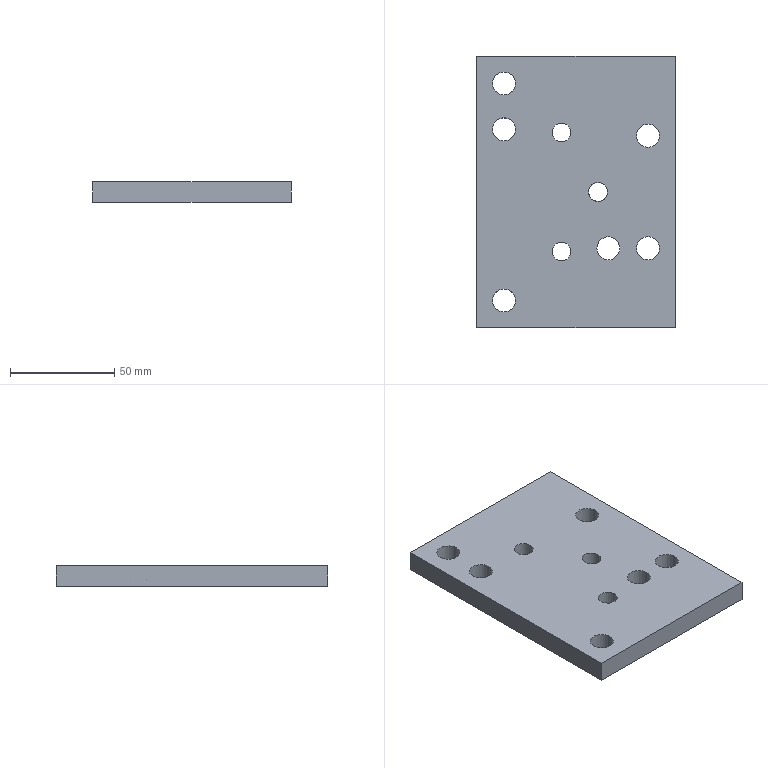Part | STEP file | PN_0042_id870_x_t | 1 solid | 15 faces | box 95 x 130 x 10 mm | volume 115889 mm3 | cylinder 9 | plane 6 | commonest cylinder face diameters 11 x6 9 x3
STEP:
#1=CARTESIAN_POINT('',(-190.55,-65.,105.));
#2=VERTEX_POINT('',#1);
#3=CARTESIAN_POINT('',(-190.55,65.,105.));
#4=VERTEX_POINT('',#3);
#5=CARTESIAN_POINT('',(-190.55,64.,105.));
#6=DIRECTION('',(0.,1.,0.));
#7=VECTOR('',#6,1.);
#8=LINE('',#5,#7);
#9=EDGE_CURVE('',#2,#4,#8,.T.);
#10=ORIENTED_EDGE('',*,*,#9,.F.);
#11=CARTESIAN_POINT('',(-190.55,-65.,95.));
#12=VERTEX_POINT('',#11);
#13=CARTESIAN_POINT('',(-190.55,-65.,95.));
#14=DIRECTION('',(0.,0.,1.));
#15=VECTOR('',#14,1.);
#16=LINE('',#13,#15);
#17=EDGE_CURVE('',#12,#2,#16,.T.);
#18=ORIENTED_EDGE('',*,*,#17,.F.);
#19=CARTESIAN_POINT('',(-190.55,65.,95.));
#20=VERTEX_POINT('',#19);
#21=CARTESIAN_POINT('',(-190.55,0.,95.));
#22=DIRECTION('',(0.,1.,0.));
#23=VECTOR('',#22,1.);
#24=LINE('',#21,#23);
#25=EDGE_CURVE('',#12,#20,#24,.T.);
#26=ORIENTED_EDGE('',*,*,#25,.T.);
#27=CARTESIAN_POINT('',(-190.55,65.,95.));
#28=DIRECTION('',(0.,0.,-1.));
#29=VECTOR('',#28,1.);
#30=LINE('',#27,#29);
#31=EDGE_CURVE('',#4,#20,#30,.T.);
#32=ORIENTED_EDGE('',*,*,#31,.F.);
#33=EDGE_LOOP('',(#10,#18,#26,#32));
#34=FACE_OUTER_BOUND('',#33,.T.);
#35=CARTESIAN_POINT('',(-190.55,0.,95.));
#36=DIRECTION('',(1.,0.,0.));
#37=DIRECTION('',(0.,1.,0.));
#38=AXIS2_PLACEMENT_3D('',#35,#36,#37);
#39=PLANE('',#38);
#40=ADVANCED_FACE('',(#34),#39,.T.);
#41=CARTESIAN_POINT('',(-285.55,-65.,95.));
#42=VERTEX_POINT('',#41);
#43=CARTESIAN_POINT('',(-224.,-65.,95.));
#44=DIRECTION('',(1.,0.,0.));
#45=VECTOR('',#44,1.);
#46=LINE('',#43,#45);
#47=EDGE_CURVE('',#42,#12,#46,.T.);
#48=ORIENTED_EDGE('',*,*,#47,.T.);
#49=ORIENTED_EDGE('',*,*,#17,.T.);
#50=CARTESIAN_POINT('',(-285.55,-65.,105.));
#51=VERTEX_POINT('',#50);
#52=CARTESIAN_POINT('',(-224.,-65.,105.));
#53=DIRECTION('',(1.,0.,0.));
#54=VECTOR('',#53,1.);
#55=LINE('',#52,#54);
#56=EDGE_CURVE('',#51,#2,#55,.T.);
#57=ORIENTED_EDGE('',*,*,#56,.F.);
#58=CARTESIAN_POINT('',(-285.55,-65.,95.));
#59=DIRECTION('',(0.,0.,1.));
#60=VECTOR('',#59,1.);
#61=LINE('',#58,#60);
#62=EDGE_CURVE('',#42,#51,#61,.T.);
#63=ORIENTED_EDGE('',*,*,#62,.F.);
#64=EDGE_LOOP('',(#48,#49,#57,#63));
#65=FACE_OUTER_BOUND('',#64,.T.);
#66=CARTESIAN_POINT('',(-224.,-65.,95.));
#67=DIRECTION('',(0.,1.,0.));
#68=DIRECTION('',(-1.,0.,0.));
#69=AXIS2_PLACEMENT_3D('',#66,#67,#68);
#70=PLANE('',#69);
#71=ADVANCED_FACE('',(#65),#70,.F.);
#72=ORIENTED_EDGE('',*,*,#9,.T.);
#73=CARTESIAN_POINT('',(-285.55,65.,105.));
#74=VERTEX_POINT('',#73);
#75=CARTESIAN_POINT('',(-119.811,65.,105.));
#76=DIRECTION('',(1.,0.,0.));
#77=VECTOR('',#76,1.);
#78=LINE('',#75,#77);
#79=EDGE_CURVE('',#74,#4,#78,.T.);
#80=ORIENTED_EDGE('',*,*,#79,.F.);
#81=CARTESIAN_POINT('',(-285.55,0.,105.));
#82=DIRECTION('',(0.,-1.,0.));
#83=VECTOR('',#82,1.);
#84=LINE('',#81,#83);
#85=EDGE_CURVE('',#74,#51,#84,.T.);
#86=ORIENTED_EDGE('',*,*,#85,.T.);
#87=ORIENTED_EDGE('',*,*,#56,.T.);
#88=EDGE_LOOP('',(#72,#80,#86,#87));
#89=FACE_BOUND('',#88,.T.);
#90=CARTESIAN_POINT('',(-228.05,-27.,105.));
#91=VERTEX_POINT('',#90);
#92=CARTESIAN_POINT('',(-222.55,-27.,105.));
#93=DIRECTION('',(0.,0.,-1.));
#94=DIRECTION('',(-1.,0.,0.));
#95=AXIS2_PLACEMENT_3D('',#92,#93,#94);
#96=CIRCLE('',#95,5.5);
#97=EDGE_CURVE('',#91,#91,#96,.T.);
#98=ORIENTED_EDGE('',*,*,#97,.T.);
#99=EDGE_LOOP('',(#98));
#100=FACE_BOUND('',#99,.T.);
#101=CARTESIAN_POINT('',(-278.05,30.,105.));
#102=VERTEX_POINT('',#101);
#103=CARTESIAN_POINT('',(-272.55,30.,105.));
#104=DIRECTION('',(0.,0.,-1.));
#105=DIRECTION('',(-1.,0.,0.));
#106=AXIS2_PLACEMENT_3D('',#103,#104,#105);
#107=CIRCLE('',#106,5.5);
#108=EDGE_CURVE('',#102,#102,#107,.T.);
#109=ORIENTED_EDGE('',*,*,#108,.T.);
#110=EDGE_LOOP('',(#109));
#111=FACE_BOUND('',#110,.T.);
#112=CARTESIAN_POINT('',(-278.05,52.,105.));
#113=VERTEX_POINT('',#112);
#114=CARTESIAN_POINT('',(-272.55,52.,105.));
#115=DIRECTION('',(0.,0.,-1.));
#116=DIRECTION('',(-1.,0.,0.));
#117=AXIS2_PLACEMENT_3D('',#114,#115,#116);
#118=CIRCLE('',#117,5.5);
#119=EDGE_CURVE('',#113,#113,#118,.T.);
#120=ORIENTED_EDGE('',*,*,#119,.T.);
#121=EDGE_LOOP('',(#120));
#122=FACE_BOUND('',#121,.T.);
#123=CARTESIAN_POINT('',(-278.05,-52.,105.));
#124=VERTEX_POINT('',#123);
#125=CARTESIAN_POINT('',(-272.55,-52.,105.));
#126=DIRECTION('',(0.,0.,1.));
#127=DIRECTION('',(-1.,0.,0.));
#128=AXIS2_PLACEMENT_3D('',#125,#126,#127);
#129=CIRCLE('',#128,5.5);
#130=EDGE_CURVE('',#124,#124,#129,.T.);
#131=ORIENTED_EDGE('',*,*,#130,.F.);
#132=EDGE_LOOP('',(#131));
#133=FACE_BOUND('',#132,.T.);
#134=CARTESIAN_POINT('',(-209.05,-27.,105.));
#135=VERTEX_POINT('',#134);
#136=CARTESIAN_POINT('',(-203.55,-27.,105.));
#137=DIRECTION('',(0.,0.,1.));
#138=DIRECTION('',(-1.,0.,0.));
#139=AXIS2_PLACEMENT_3D('',#136,#137,#138);
#140=CIRCLE('',#139,5.5);
#141=EDGE_CURVE('',#135,#135,#140,.T.);
#142=ORIENTED_EDGE('',*,*,#141,.F.);
#143=EDGE_LOOP('',(#142));
#144=FACE_BOUND('',#143,.T.);
#145=CARTESIAN_POINT('',(-209.05,27.,105.));
#146=VERTEX_POINT('',#145);
#147=CARTESIAN_POINT('',(-203.55,27.,105.));
#148=DIRECTION('',(0.,0.,-1.));
#149=DIRECTION('',(-1.,0.,0.));
#150=AXIS2_PLACEMENT_3D('',#147,#148,#149);
#151=CIRCLE('',#150,5.5);
#152=EDGE_CURVE('',#146,#146,#151,.T.);
#153=ORIENTED_EDGE('',*,*,#152,.T.);
#154=EDGE_LOOP('',(#153));
#155=FACE_BOUND('',#154,.T.);
#156=CARTESIAN_POINT('',(-227.5,4.5,105.));
#157=VERTEX_POINT('',#156);
#158=CARTESIAN_POINT('',(-227.5,0.,105.));
#159=DIRECTION('',(0.,0.,-1.));
#160=DIRECTION('',(0.,1.,0.));
#161=AXIS2_PLACEMENT_3D('',#158,#159,#160);
#162=CIRCLE('',#161,4.5);
#163=EDGE_CURVE('',#157,#157,#162,.T.);
#164=ORIENTED_EDGE('',*,*,#163,.T.);
#165=EDGE_LOOP('',(#164));
#166=FACE_BOUND('',#165,.T.);
#167=CARTESIAN_POINT('',(-249.5,-28.5,105.));
#168=VERTEX_POINT('',#167);
#169=CARTESIAN_POINT('',(-245.,-28.5,105.));
#170=DIRECTION('',(0.,0.,1.));
#171=DIRECTION('',(-1.,0.,0.));
#172=AXIS2_PLACEMENT_3D('',#169,#170,#171);
#173=CIRCLE('',#172,4.5);
#174=EDGE_CURVE('',#168,#168,#173,.T.);
#175=ORIENTED_EDGE('',*,*,#174,.F.);
#176=EDGE_LOOP('',(#175));
#177=FACE_BOUND('',#176,.T.);
#178=CARTESIAN_POINT('',(-249.5,28.5,105.));
#179=VERTEX_POINT('',#178);
#180=CARTESIAN_POINT('',(-245.,28.5,105.));
#181=DIRECTION('',(0.,0.,-1.));
#182=DIRECTION('',(-1.,0.,0.));
#183=AXIS2_PLACEMENT_3D('',#180,#181,#182);
#184=CIRCLE('',#183,4.5);
#185=EDGE_CURVE('',#179,#179,#184,.T.);
#186=ORIENTED_EDGE('',*,*,#185,.T.);
#187=EDGE_LOOP('',(#186));
#188=FACE_BOUND('',#187,.T.);
#189=CARTESIAN_POINT('',(-119.811,64.,105.));
#190=DIRECTION('',(0.,0.,1.));
#191=DIRECTION('',(1.,0.,0.));
#192=AXIS2_PLACEMENT_3D('',#189,#190,#191);
#193=PLANE('',#192);
#194=ADVANCED_FACE('',(#89,#100,#111,#122,#133,#144,#155,#166,#177,#188),#193,.T.);
#195=ORIENTED_EDGE('',*,*,#25,.F.);
#196=ORIENTED_EDGE('',*,*,#47,.F.);
#197=CARTESIAN_POINT('',(-285.55,65.,95.));
#198=VERTEX_POINT('',#197);
#199=CARTESIAN_POINT('',(-285.55,0.,95.));
#200=DIRECTION('',(0.,-1.,0.));
#201=VECTOR('',#200,1.);
#202=LINE('',#199,#201);
#203=EDGE_CURVE('',#198,#42,#202,.T.);
#204=ORIENTED_EDGE('',*,*,#203,.F.);
#205=CARTESIAN_POINT('',(-119.811,65.,95.));
#206=DIRECTION('',(1.,0.,0.));
#207=VECTOR('',#206,1.);
#208=LINE('',#205,#207);
#209=EDGE_CURVE('',#198,#20,#208,.T.);
#210=ORIENTED_EDGE('',*,*,#209,.T.);
#211=EDGE_LOOP('',(#195,#196,#204,#210));
#212=FACE_BOUND('',#211,.T.);
#213=CARTESIAN_POINT('',(-228.05,-27.,95.));
#214=VERTEX_POINT('',#213);
#215=CARTESIAN_POINT('',(-222.55,-27.,95.));
#216=DIRECTION('',(0.,0.,1.));
#217=DIRECTION('',(-1.,0.,0.));
#218=AXIS2_PLACEMENT_3D('',#215,#216,#217);
#219=CIRCLE('',#218,5.5);
#220=EDGE_CURVE('',#214,#214,#219,.T.);
#221=ORIENTED_EDGE('',*,*,#220,.T.);
#222=EDGE_LOOP('',(#221));
#223=FACE_BOUND('',#222,.T.);
#224=CARTESIAN_POINT('',(-278.05,30.,95.));
#225=VERTEX_POINT('',#224);
#226=CARTESIAN_POINT('',(-272.55,30.,95.));
#227=DIRECTION('',(0.,0.,1.));
#228=DIRECTION('',(-1.,0.,0.));
#229=AXIS2_PLACEMENT_3D('',#226,#227,#228);
#230=CIRCLE('',#229,5.5);
#231=EDGE_CURVE('',#225,#225,#230,.T.);
#232=ORIENTED_EDGE('',*,*,#231,.T.);
#233=EDGE_LOOP('',(#232));
#234=FACE_BOUND('',#233,.T.);
#235=CARTESIAN_POINT('',(-267.05,52.,95.));
#236=VERTEX_POINT('',#235);
#237=CARTESIAN_POINT('',(-272.55,52.,95.));
#238=DIRECTION('',(0.,0.,-1.));
#239=DIRECTION('',(1.,0.,0.));
#240=AXIS2_PLACEMENT_3D('',#237,#238,#239);
#241=CIRCLE('',#240,5.5);
#242=EDGE_CURVE('',#236,#236,#241,.T.);
#243=ORIENTED_EDGE('',*,*,#242,.F.);
#244=EDGE_LOOP('',(#243));
#245=FACE_BOUND('',#244,.T.);
#246=CARTESIAN_POINT('',(-267.05,-52.,95.));
#247=VERTEX_POINT('',#246);
#248=CARTESIAN_POINT('',(-272.55,-52.,95.));
#249=DIRECTION('',(0.,0.,-1.));
#250=DIRECTION('',(1.,0.,0.));
#251=AXIS2_PLACEMENT_3D('',#248,#249,#250);
#252=CIRCLE('',#251,5.5);
#253=EDGE_CURVE('',#247,#247,#252,.T.);
#254=ORIENTED_EDGE('',*,*,#253,.F.);
#255=EDGE_LOOP('',(#254));
#256=FACE_BOUND('',#255,.T.);
#257=CARTESIAN_POINT('',(-198.05,-27.,95.));
#258=VERTEX_POINT('',#257);
#259=CARTESIAN_POINT('',(-203.55,-27.,95.));
#260=DIRECTION('',(0.,0.,-1.));
#261=DIRECTION('',(1.,0.,0.));
#262=AXIS2_PLACEMENT_3D('',#259,#260,#261);
#263=CIRCLE('',#262,5.5);
#264=EDGE_CURVE('',#258,#258,#263,.T.);
#265=ORIENTED_EDGE('',*,*,#264,.F.);
#266=EDGE_LOOP('',(#265));
#267=FACE_BOUND('',#266,.T.);
#268=CARTESIAN_POINT('',(-198.05,27.,95.));
#269=VERTEX_POINT('',#268);
#270=CARTESIAN_POINT('',(-203.55,27.,95.));
#271=DIRECTION('',(0.,0.,-1.));
#272=DIRECTION('',(1.,0.,0.));
#273=AXIS2_PLACEMENT_3D('',#270,#271,#272);
#274=CIRCLE('',#273,5.5);
#275=EDGE_CURVE('',#269,#269,#274,.T.);
#276=ORIENTED_EDGE('',*,*,#275,.F.);
#277=EDGE_LOOP('',(#276));
#278=FACE_BOUND('',#277,.T.);
#279=CARTESIAN_POINT('',(-223.,0.,95.));
#280=VERTEX_POINT('',#279);
#281=CARTESIAN_POINT('',(-227.5,0.,95.));
#282=DIRECTION('',(0.,0.,-1.));
#283=DIRECTION('',(1.,0.,0.));
#284=AXIS2_PLACEMENT_3D('',#281,#282,#283);
#285=CIRCLE('',#284,4.5);
#286=EDGE_CURVE('',#280,#280,#285,.T.);
#287=ORIENTED_EDGE('',*,*,#286,.F.);
#288=EDGE_LOOP('',(#287));
#289=FACE_BOUND('',#288,.T.);
#290=CARTESIAN_POINT('',(-240.5,-28.5,95.));
#291=VERTEX_POINT('',#290);
#292=CARTESIAN_POINT('',(-245.,-28.5,95.));
#293=DIRECTION('',(0.,0.,-1.));
#294=DIRECTION('',(1.,0.,0.));
#295=AXIS2_PLACEMENT_3D('',#292,#293,#294);
#296=CIRCLE('',#295,4.5);
#297=EDGE_CURVE('',#291,#291,#296,.T.);
#298=ORIENTED_EDGE('',*,*,#297,.F.);
#299=EDGE_LOOP('',(#298));
#300=FACE_BOUND('',#299,.T.);
#301=CARTESIAN_POINT('',(-240.5,28.5,95.));
#302=VERTEX_POINT('',#301);
#303=CARTESIAN_POINT('',(-245.,28.5,95.));
#304=DIRECTION('',(0.,0.,-1.));
#305=DIRECTION('',(1.,0.,0.));
#306=AXIS2_PLACEMENT_3D('',#303,#304,#305);
#307=CIRCLE('',#306,4.5);
#308=EDGE_CURVE('',#302,#302,#307,.T.);
#309=ORIENTED_EDGE('',*,*,#308,.F.);
#310=EDGE_LOOP('',(#309));
#311=FACE_BOUND('',#310,.T.);
#312=CARTESIAN_POINT('',(-119.811,64.,95.));
#313=DIRECTION('',(0.,0.,1.));
#314=DIRECTION('',(1.,0.,0.));
#315=AXIS2_PLACEMENT_3D('',#312,#313,#314);
#316=PLANE('',#315);
#317=ADVANCED_FACE('',(#212,#223,#234,#245,#256,#267,#278,#289,#300,#311),#316,.F.);
#318=CARTESIAN_POINT('',(-285.55,65.,95.));
#319=DIRECTION('',(0.,0.,1.));
#320=VECTOR('',#319,1.);
#321=LINE('',#318,#320);
#322=EDGE_CURVE('',#198,#74,#321,.T.);
#323=ORIENTED_EDGE('',*,*,#322,.F.);
#324=ORIENTED_EDGE('',*,*,#203,.T.);
#325=ORIENTED_EDGE('',*,*,#62,.T.);
#326=ORIENTED_EDGE('',*,*,#85,.F.);
#327=EDGE_LOOP('',(#323,#324,#325,#326));
#328=FACE_OUTER_BOUND('',#327,.T.);
#329=CARTESIAN_POINT('',(-285.55,0.,95.));
#330=DIRECTION('',(1.,0.,0.));
#331=DIRECTION('',(0.,1.,0.));
#332=AXIS2_PLACEMENT_3D('',#329,#330,#331);
#333=PLANE('',#332);
#334=ADVANCED_FACE('',(#328),#333,.F.);
#335=ORIENTED_EDGE('',*,*,#79,.T.);
#336=ORIENTED_EDGE('',*,*,#31,.T.);
#337=ORIENTED_EDGE('',*,*,#209,.F.);
#338=ORIENTED_EDGE('',*,*,#322,.T.);
#339=EDGE_LOOP('',(#335,#336,#337,#338));
#340=FACE_OUTER_BOUND('',#339,.T.);
#341=CARTESIAN_POINT('',(-119.811,65.,95.));
#342=DIRECTION('',(0.,-1.,0.));
#343=DIRECTION('',(1.,0.,0.));
#344=AXIS2_PLACEMENT_3D('',#341,#342,#343);
#345=PLANE('',#344);
#346=ADVANCED_FACE('',(#340),#345,.F.);
#347=ORIENTED_EDGE('',*,*,#308,.T.);
#348=EDGE_LOOP('',(#347));
#349=FACE_BOUND('',#348,.T.);
#350=ORIENTED_EDGE('',*,*,#185,.F.);
#351=EDGE_LOOP('',(#350));
#352=FACE_BOUND('',#351,.T.);
#353=CARTESIAN_POINT('',(-245.,28.5,105.));
#354=DIRECTION('',(0.,0.,-1.));
#355=DIRECTION('',(-1.,0.,0.));
#356=AXIS2_PLACEMENT_3D('',#353,#354,#355);
#357=CYLINDRICAL_SURFACE('',#356,4.5);
#358=ADVANCED_FACE('',(#349,#352),#357,.F.);
#359=ORIENTED_EDGE('',*,*,#297,.T.);
#360=EDGE_LOOP('',(#359));
#361=FACE_BOUND('',#360,.T.);
#362=ORIENTED_EDGE('',*,*,#174,.T.);
#363=EDGE_LOOP('',(#362));
#364=FACE_BOUND('',#363,.T.);
#365=CARTESIAN_POINT('',(-245.,-28.5,105.));
#366=DIRECTION('',(0.,0.,-1.));
#367=DIRECTION('',(-1.,0.,0.));
#368=AXIS2_PLACEMENT_3D('',#365,#366,#367);
#369=CYLINDRICAL_SURFACE('',#368,4.5);
#370=ADVANCED_FACE('',(#361,#364),#369,.F.);
#371=ORIENTED_EDGE('',*,*,#286,.T.);
#372=EDGE_LOOP('',(#371));
#373=FACE_BOUND('',#372,.T.);
#374=ORIENTED_EDGE('',*,*,#163,.F.);
#375=EDGE_LOOP('',(#374));
#376=FACE_BOUND('',#375,.T.);
#377=CARTESIAN_POINT('',(-227.5,0.,105.));
#378=DIRECTION('',(0.,0.,-1.));
#379=DIRECTION('',(0.,1.,0.));
#380=AXIS2_PLACEMENT_3D('',#377,#378,#379);
#381=CYLINDRICAL_SURFACE('',#380,4.5);
#382=ADVANCED_FACE('',(#373,#376),#381,.F.);
#383=ORIENTED_EDGE('',*,*,#275,.T.);
#384=EDGE_LOOP('',(#383));
#385=FACE_BOUND('',#384,.T.);
#386=ORIENTED_EDGE('',*,*,#152,.F.);
#387=EDGE_LOOP('',(#386));
#388=FACE_BOUND('',#387,.T.);
#389=CARTESIAN_POINT('',(-203.55,27.,105.));
#390=DIRECTION('',(0.,0.,-1.));
#391=DIRECTION('',(-1.,0.,0.));
#392=AXIS2_PLACEMENT_3D('',#389,#390,#391);
#393=CYLINDRICAL_SURFACE('',#392,5.5);
#394=ADVANCED_FACE('',(#385,#388),#393,.F.);
#395=ORIENTED_EDGE('',*,*,#264,.T.);
#396=EDGE_LOOP('',(#395));
#397=FACE_BOUND('',#396,.T.);
#398=ORIENTED_EDGE('',*,*,#141,.T.);
#399=EDGE_LOOP('',(#398));
#400=FACE_BOUND('',#399,.T.);
#401=CARTESIAN_POINT('',(-203.55,-27.,105.));
#402=DIRECTION('',(0.,0.,-1.));
#403=DIRECTION('',(-1.,0.,0.));
#404=AXIS2_PLACEMENT_3D('',#401,#402,#403);
#405=CYLINDRICAL_SURFACE('',#404,5.5);
#406=ADVANCED_FACE('',(#397,#400),#405,.F.);
#407=ORIENTED_EDGE('',*,*,#253,.T.);
#408=EDGE_LOOP('',(#407));
#409=FACE_BOUND('',#408,.T.);
#410=ORIENTED_EDGE('',*,*,#130,.T.);
#411=EDGE_LOOP('',(#410));
#412=FACE_BOUND('',#411,.T.);
#413=CARTESIAN_POINT('',(-272.55,-52.,105.));
#414=DIRECTION('',(0.,0.,-1.));
#415=DIRECTION('',(-1.,0.,0.));
#416=AXIS2_PLACEMENT_3D('',#413,#414,#415);
#417=CYLINDRICAL_SURFACE('',#416,5.5);
#418=ADVANCED_FACE('',(#409,#412),#417,.F.);
#419=ORIENTED_EDGE('',*,*,#242,.T.);
#420=EDGE_LOOP('',(#419));
#421=FACE_BOUND('',#420,.T.);
#422=ORIENTED_EDGE('',*,*,#119,.F.);
#423=EDGE_LOOP('',(#422));
#424=FACE_BOUND('',#423,.T.);
#425=CARTESIAN_POINT('',(-272.55,52.,105.));
#426=DIRECTION('',(0.,0.,-1.));
#427=DIRECTION('',(-1.,0.,0.));
#428=AXIS2_PLACEMENT_3D('',#425,#426,#427);
#429=CYLINDRICAL_SURFACE('',#428,5.5);
#430=ADVANCED_FACE('',(#421,#424),#429,.F.);
#431=ORIENTED_EDGE('',*,*,#231,.F.);
#432=EDGE_LOOP('',(#431));
#433=FACE_BOUND('',#432,.T.);
#434=ORIENTED_EDGE('',*,*,#108,.F.);
#435=EDGE_LOOP('',(#434));
#436=FACE_BOUND('',#435,.T.);
#437=CARTESIAN_POINT('',(-272.55,30.,105.));
#438=DIRECTION('',(0.,0.,-1.));
#439=DIRECTION('',(-1.,0.,0.));
#440=AXIS2_PLACEMENT_3D('',#437,#438,#439);
#441=CYLINDRICAL_SURFACE('',#440,5.5);
#442=ADVANCED_FACE('',(#433,#436),#441,.F.);
#443=ORIENTED_EDGE('',*,*,#220,.F.);
#444=EDGE_LOOP('',(#443));
#445=FACE_BOUND('',#444,.T.);
#446=ORIENTED_EDGE('',*,*,#97,.F.);
#447=EDGE_LOOP('',(#446));
#448=FACE_BOUND('',#447,.T.);
#449=CARTESIAN_POINT('',(-222.55,-27.,105.));
#450=DIRECTION('',(0.,0.,-1.));
#451=DIRECTION('',(-1.,0.,0.));
#452=AXIS2_PLACEMENT_3D('',#449,#450,#451);
#453=CYLINDRICAL_SURFACE('',#452,5.5);
#454=ADVANCED_FACE('',(#445,#448),#453,.F.);
#455=CLOSED_SHELL('',(#40,#71,#194,#317,#334,#346,#358,#370,#382,#394,#406,#418,#430,#442,#454));
#456=MANIFOLD_SOLID_BREP('',#455);
#457=(LENGTH_UNIT()NAMED_UNIT(*)SI_UNIT(.MILLI.,.METRE.));
#458=UNCERTAINTY_MEASURE_WITH_UNIT(LENGTH_MEASURE(0.00002),#457,'','');
#459=(NAMED_UNIT(*)PLANE_ANGLE_UNIT()SI_UNIT($,.RADIAN.));
#460=PLANE_ANGLE_MEASURE_WITH_UNIT(PLANE_ANGLE_MEASURE(0.01745),#459);
#461=DIMENSIONAL_EXPONENTS(0.,0.,0.,0.,0.,0.,0.);
#462=(CONVERSION_BASED_UNIT('DEGREE',#460)NAMED_UNIT(#461)PLANE_ANGLE_UNIT());
#463=(NAMED_UNIT(*)SI_UNIT($,.STERADIAN.)SOLID_ANGLE_UNIT());
#464=(GEOMETRIC_REPRESENTATION_CONTEXT(3)GLOBAL_UNCERTAINTY_ASSIGNED_CONTEXT((#458))GLOBAL_UNIT_ASSIGNED_CONTEXT((#457,#462,#463))REPRESENTATION_CONTEXT('',''));
#465=ADVANCED_BREP_SHAPE_REPRESENTATION('',(#456),#464);